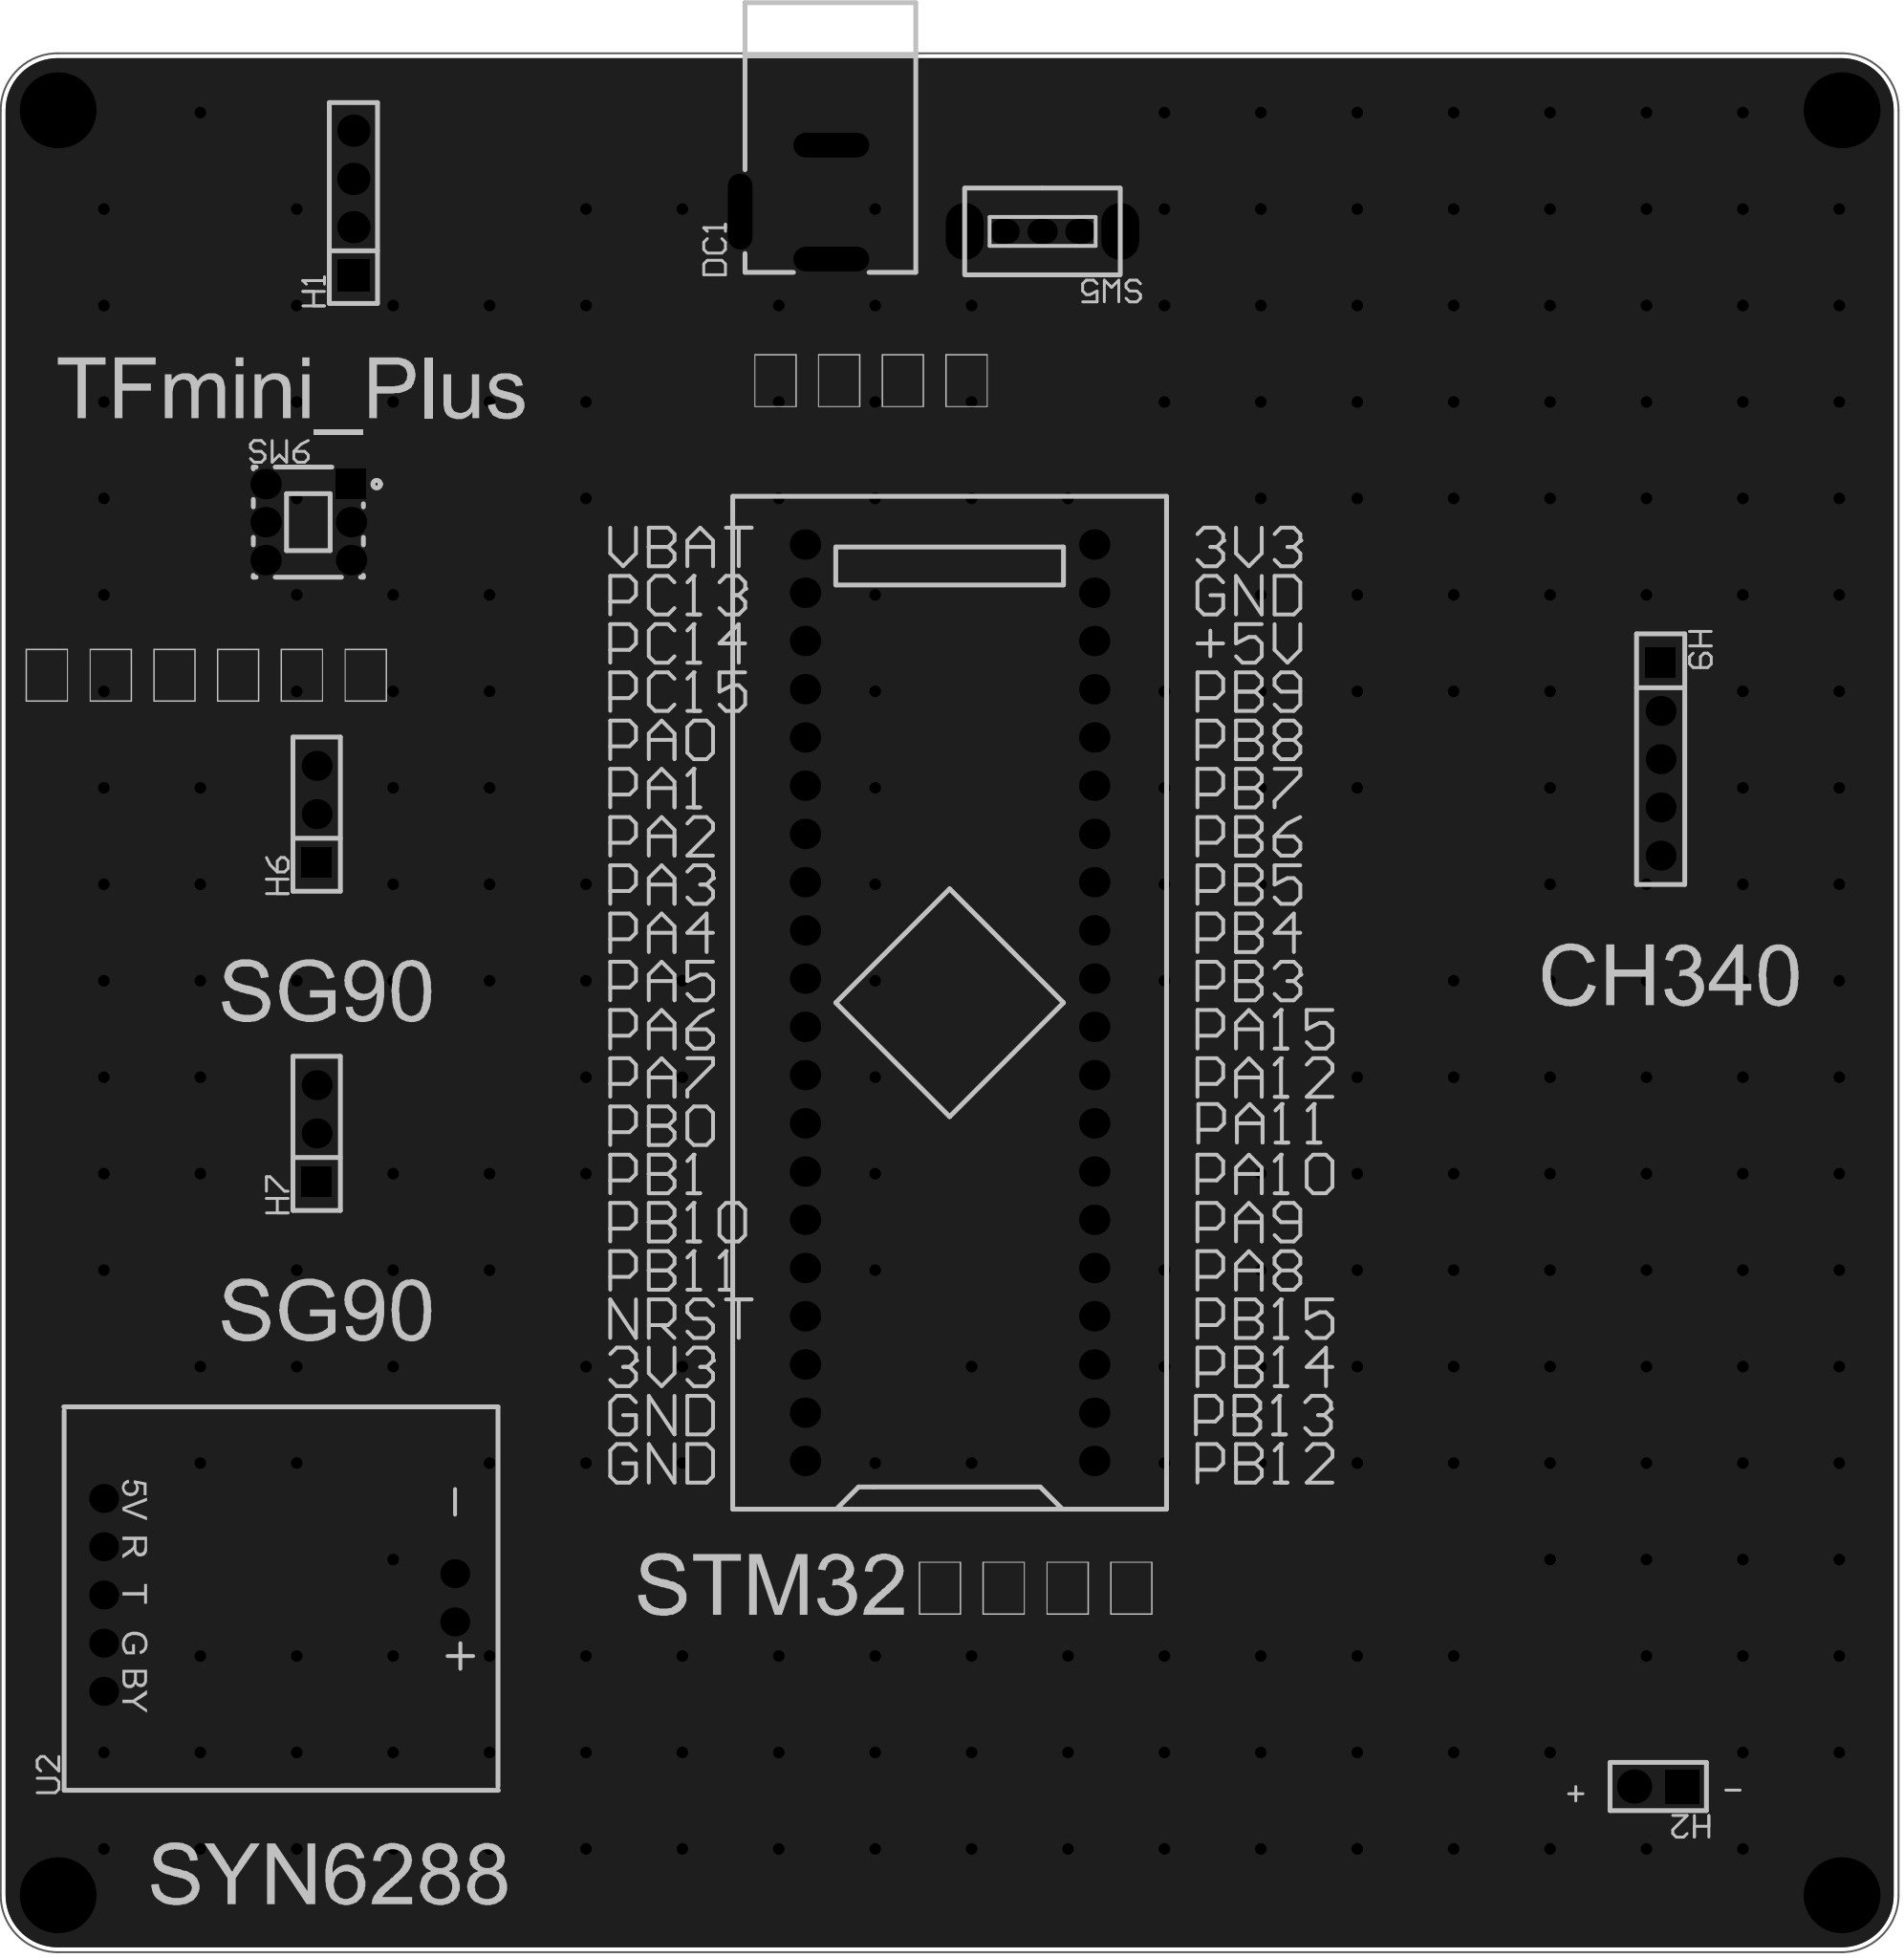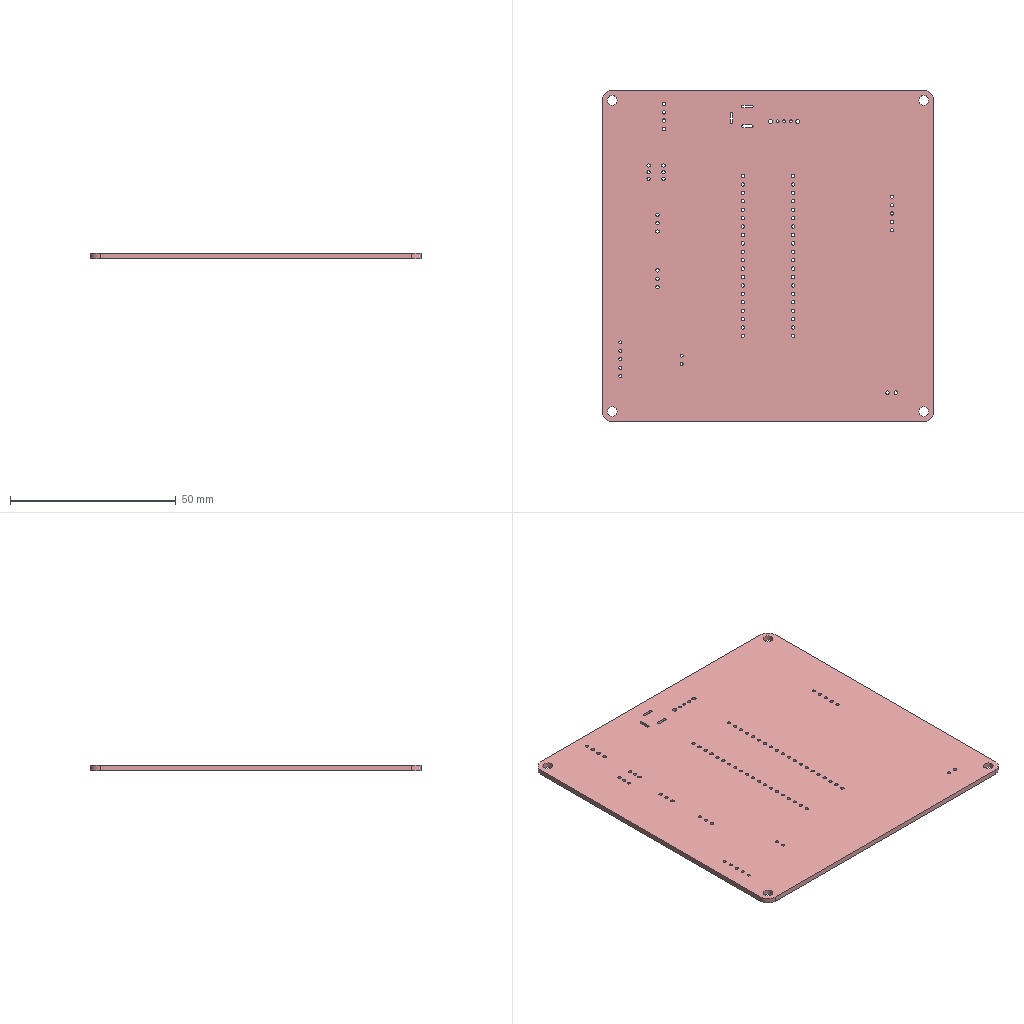Circuit board layout | Altium Designer | box 100 x 100 x 1.6 mm
Layer stack:
# Altium Designer layer stack of  (unit mm; dielectric type: 0 none, 1 core, 2 prepreg, 3 surface material)
index,name,kind,layer,copper_thickness_mm,dielectric_type,dielectric_thickness_mm,dielectric_material,dielectric_constant
0,Top Paste Mask Layer,other,,,,,,
1,Top Silkscreen Layer,other,,,,,,
2,Top Solder Mask Layer,dielectric,,,3,0.01,,3.3
3,Top Layer,copper,Top Layer,0.035,,,,
4,Dielectric1,dielectric,,,3,1.51,FR4,4.5
5,Bottom Layer,copper,Bottom Layer,0.035,,,,
6,Bottom Solder Mask Layer,dielectric,,,3,0.01,,3.3
7,Bottom Silkscreen Layer,other,,,,,,
8,Bottom Paste Mask Layer,other,,,,,,
# drill layer pairs: low layer,high layer
drill_pair,Top Layer,Bottom Layer
Part placement:
Designator,Comment,Layer,Footprint,Center-X(mm),Center-Y(mm),Rotation
U1,STM32F103C8T6-Card,TopLayer,CONN-TH_L53.3-W22.9_STM32F103C8T6-CARD,141.351,130.937,90
H6,,TopLayer,HDR-TH_3P-P2.54-V-F,107.999,140.868,90
H7,,TopLayer,HDR-TH_3P-P2.54-V-F,107.999,124.057,90
H9,,TopLayer,HDR-TH_5P-P2.54-V-F,178.816,143.764,270
SW5,,TopLayer,拨动开关,146.243,171.555,180
SW6,TK-6580-1,TopLayer,SW-TH_TK-6580-1,107.561,156.247,0
H1,,TopLayer,HDR-TH_4P-P2.54-V-F,109.936,173.052,90
H2,,TopLayer,HDR-TH_2P-P2.54-V-M-1,178.689,89.662,180
U2,SYN6288,TopLayer,SYN6288,106.025,99.75,90
DC1,,TopLayer,DC-2.0,132.715,173.101,90
Pad and via stacks:
# Altium Designer via and pad stacks of  (unit mm). Each distinct definition once, with the count of objects using it.
# via: kind,start_layer,end_layer,hole_mm,diameter_mm,mode(0 simple;1 top-mid-bottom;2 full stack),diameter_per_layer,count,example_net
# pad: kind,layer,hole_mm,hole_type(0 round;1 square;2 slot),plating,top_size,top_shape(1 round;2 rect;3 octagon;9 rounded rect),mid_size,bottom_size,mode,footprint,size_per_layer,count,example
pad,Multi-Layer,3,0,plated,4x4,1,4x4,4x4,0,,,4,1
pad,Multi-Layer,1,0,plated,1.6x1.6,1,1.6x1.6,1.6x1.6,0,CONN-TH_L53.3-W22.9_STM32F103C8T6-CARD,,40,U1.1
pad,Multi-Layer,1.02,0,plated,1.575x1.575,1,1.575x1.575,1.575x1.575,0,HDR-TH_3P-P2.54-V-F,,4,H6.3
pad,Multi-Layer,1.02,0,plated,1.575x1.575,2,1.575x1.575,1.575x1.575,0,HDR-TH_3P-P2.54-V-F,,2,H6.1
pad,Multi-Layer,1.02,0,plated,1.575x1.575,1,1.575x1.575,1.575x1.575,0,HDR-TH_5P-P2.54-V-F,,4,H9.5
pad,Multi-Layer,1.02,0,plated,1.575x1.575,2,1.575x1.575,1.575x1.575,0,HDR-TH_5P-P2.54-V-F,,1,H9.1
pad,Multi-Layer,0.8992,0,plated,1.6x1.3,1,1.6x1.3,1.6x1.3,0,\u00B2\u00A6\u00B6\u00AF\u00BF\u00AA\u00B9\u00D8,,3,SW5.1
pad,Multi-Layer,1.3,0,plated,3x1.999,1,3x1.999,3x1.999,0,\u00B2\u00A6\u00B6\u00AF\u00BF\u00AA\u00B9\u00D8,,2,SW5.4
pad,Multi-Layer,1,0,plated,1.6x1.6,2,1.6x1.6,1.6x1.6,0,SW-TH_TK-6580-1,,1,SW6.1
pad,Multi-Layer,1,0,plated,1.6x1.6,1,1.6x1.6,1.6x1.6,0,SW-TH_TK-6580-1,,5,SW6.2
pad,Multi-Layer,1.1,0,plated,1.7x1.7,2,1.7x1.7,1.7x1.7,0,HDR-TH_4P-P2.54-V-F,,1,H1.1
pad,Multi-Layer,1.1,0,plated,1.7x1.7,1,1.7x1.7,1.7x1.7,0,HDR-TH_4P-P2.54-V-F,,3,H1.2
pad,Multi-Layer,1.1,0,plated,1.8x1.8,1,1.8x1.8,1.8x1.8,0,HDR-TH_2P-P2.54-V-M-1,,1,H2.2
pad,Multi-Layer,1.1,0,plated,1.8x1.8,2,1.8x1.8,1.8x1.8,0,HDR-TH_2P-P2.54-V-M-1,,1,H2.1
pad,Multi-Layer,0.9144,0,plated,1.524x1.524,1,1.524x1.524,1.524x1.524,0,SYN6288,,7,U2.5
pad,Multi-Layer,0.8001,2,plated,4x1.3,1,4x1.3,4x1.3,0,DC-2.0,,3,DC1.2
via,Top Layer,Bottom Layer,0.3048,0.61,0,,252,GND
Copper pours:
name,layer,net,type(0 solid;1 hatched;2 none)
Bottom Layer-GND,Bottom Layer,GND,0
Top Layer-GND,Top Layer,GND,0
Design rules, without the lines most boards share:
# Altium Designer design rules of  (exported by Altium Designer, unit mm)
# columns: name | kind | enabled | priority | scope1 | scope2 | descriptor | typed fields (field=value)
Copper_copperRegion_copperThickness1oz | 0 | disabled | 4 | All | All | Clearance Constraint (Gap=5.984mil) (Disabled)(All),(All) | gap=0.152
Copper_copperRegion_copperThickness1oz_1 | 63 | disabled | 4 | All | All | Board Clearance Constraint (Gap=0mil) (Disabled)(All) |
Copper_copperRegion_Copper_copperRegion | 0 | disabled | 5 | All | All | Clearance Constraint (Gap=5.984mil) (Disabled)(All),(All) | gap=0.152
Copper_copperRegion_Copper_copperRegion_1 | 63 | disabled | 5 | All | All | Board Clearance Constraint (Gap=0mil) (Disabled)(All) |
copperThickness1oz | 0 | enabled | 6 | All | All | Clearance Constraint (Gap=5.984mil) (All),(All) | gap=0.152
copperThickness1oz_1 | 63 | enabled | 6 | All | All | Board Clearance Constraint (Gap=0mil) (All) |
copperRegion_copperThickness1oz | 20 | disabled | 1 | All | All | Polygon Connect Rule(Relief Connect )(Conductor Width=10mil) (Relief Angle=90 Angle) (Entries=4) (Air Gap Width=10mil) (Disabled)(All),(All) | connect_style(0=relief,1=direct,2=none)=0 relief_conductor_width=0.254 relief_entries=4
copperRegion_Copper_copperRegion | 20 | disabled | 2 | All | All | Polygon Connect Rule(Relief Connect )(Conductor Width=10mil) (Relief Angle=90 Angle) (Entries=4) (Air Gap Width=10mil) (Disabled)(All),(All) | connect_style(0=relief,1=direct,2=none)=0 relief_conductor_width=0.254 relief_entries=4
copperRegion | 20 | enabled | 3 | All | All | Polygon Connect Rule(Relief Connect )(Conductor Width=10mil) (Relief Angle=90 Angle) (Entries=4) (Air Gap Width=10mil) (All),(All) | connect_style(0=relief,1=direct,2=none)=0 relief_conductor_width=0.254 relief_entries=4